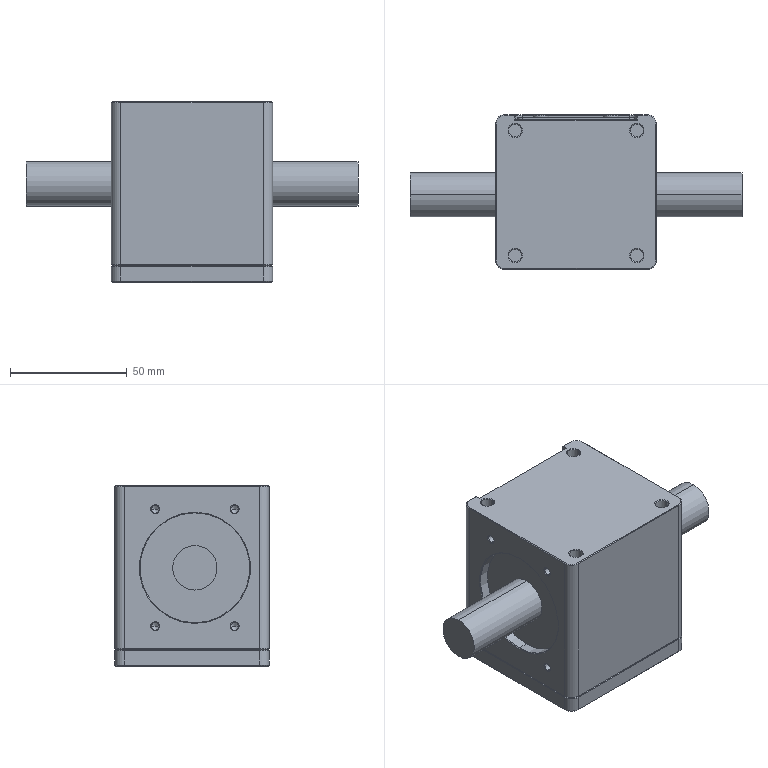Part | SolidWorks | features BaseBody 2 | 2 solids | 290 faces | box 142 x 66.1 x 77 mm | volume 347121 mm3 | plane 110 | cone 86 | cylinder 82 | spline 12 | commonest cylinder face diameters 3.3 x16 5.5 x16 3.4 x8 6.5 x8 8 x8 10 x8